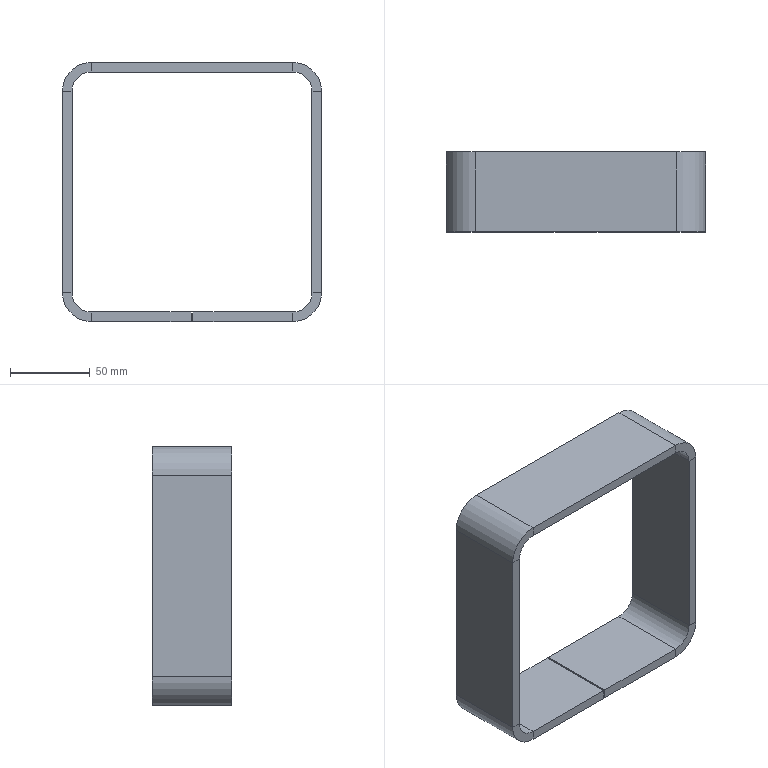Part | SolidWorks | features FlatPattern 1, SMBaseFlange 1, SheetMetal 1 | 1 solid | 38 faces | box 162 x 50 x 162 mm | volume 179174 mm3 | plane 30 | cylinder 8 | commonest cylinder face diameters 24 x4 36 x4
STEP:
#1=CARTESIAN_POINT('',(-63.,25.,-81.));
#2=VERTEX_POINT('',#1);
#3=CARTESIAN_POINT('',(-63.,25.,-75.));
#4=VERTEX_POINT('',#3);
#5=CARTESIAN_POINT('',(-63.,25.,-81.));
#6=DIRECTION('',(0.,0.,1.));
#7=VECTOR('',#6,1000.);
#8=LINE('',#5,#7);
#9=EDGE_CURVE('',#2,#4,#8,.T.);
#10=ORIENTED_EDGE('',*,*,#9,.F.);
#11=CARTESIAN_POINT('',(-81.,25.,-63.));
#12=VERTEX_POINT('',#11);
#13=CARTESIAN_POINT('',(-63.,25.,-63.));
#14=DIRECTION('',(0.,-1.,0.));
#15=DIRECTION('',(0.,0.,1.));
#16=AXIS2_PLACEMENT_3D('',#13,#14,#15);
#17=CIRCLE('',#16,18.);
#18=EDGE_CURVE('',#12,#2,#17,.T.);
#19=ORIENTED_EDGE('',*,*,#18,.F.);
#20=CARTESIAN_POINT('',(-75.,25.,-63.));
#21=VERTEX_POINT('',#20);
#22=CARTESIAN_POINT('',(-75.,25.,-63.));
#23=DIRECTION('',(-1.,0.,0.));
#24=VECTOR('',#23,1000.);
#25=LINE('',#22,#24);
#26=EDGE_CURVE('',#21,#12,#25,.T.);
#27=ORIENTED_EDGE('',*,*,#26,.F.);
#28=CARTESIAN_POINT('',(-63.,25.,-63.));
#29=DIRECTION('',(0.,-1.,0.));
#30=DIRECTION('',(1.,0.,0.));
#31=AXIS2_PLACEMENT_3D('',#28,#29,#30);
#32=CIRCLE('',#31,12.);
#33=EDGE_CURVE('',#21,#4,#32,.T.);
#34=ORIENTED_EDGE('',*,*,#33,.T.);
#35=EDGE_LOOP('',(#10,#19,#27,#34));
#36=FACE_OUTER_BOUND('',#35,.T.);
#37=CARTESIAN_POINT('',(-63.,25.,-81.));
#38=DIRECTION('',(0.,1.,0.));
#39=DIRECTION('',(0.,0.,1.));
#40=AXIS2_PLACEMENT_3D('',#37,#38,#39);
#41=PLANE('',#40);
#42=ADVANCED_FACE('',(#36),#41,.T.);
#43=CARTESIAN_POINT('',(-0.5,25.,-81.));
#44=VERTEX_POINT('',#43);
#45=CARTESIAN_POINT('',(-63.,25.,-81.));
#46=DIRECTION('',(1.,0.,0.));
#47=VECTOR('',#46,1000.);
#48=LINE('',#45,#47);
#49=EDGE_CURVE('',#2,#44,#48,.T.);
#50=ORIENTED_EDGE('',*,*,#49,.F.);
#51=ORIENTED_EDGE('',*,*,#9,.T.);
#52=CARTESIAN_POINT('',(-0.5,25.,-75.));
#53=VERTEX_POINT('',#52);
#54=CARTESIAN_POINT('',(-63.,25.,-75.));
#55=DIRECTION('',(1.,0.,0.));
#56=VECTOR('',#55,1000.);
#57=LINE('',#54,#56);
#58=EDGE_CURVE('',#4,#53,#57,.T.);
#59=ORIENTED_EDGE('',*,*,#58,.T.);
#60=CARTESIAN_POINT('',(-0.5,25.,-81.));
#61=DIRECTION('',(0.,0.,1.));
#62=VECTOR('',#61,1000.);
#63=LINE('',#60,#62);
#64=EDGE_CURVE('',#44,#53,#63,.T.);
#65=ORIENTED_EDGE('',*,*,#64,.F.);
#66=EDGE_LOOP('',(#50,#51,#59,#65));
#67=FACE_OUTER_BOUND('',#66,.T.);
#68=CARTESIAN_POINT('',(-75.,25.,-63.));
#69=DIRECTION('',(0.,1.,0.));
#70=DIRECTION('',(0.,0.,1.));
#71=AXIS2_PLACEMENT_3D('',#68,#69,#70);
#72=PLANE('',#71);
#73=ADVANCED_FACE('',(#67),#72,.T.);
#74=CARTESIAN_POINT('',(-81.,-25.,-63.));
#75=VERTEX_POINT('',#74);
#76=CARTESIAN_POINT('',(-75.,-25.,-63.));
#77=VERTEX_POINT('',#76);
#78=CARTESIAN_POINT('',(-81.,-25.,-63.));
#79=DIRECTION('',(1.,0.,0.));
#80=VECTOR('',#79,1000.);
#81=LINE('',#78,#80);
#82=EDGE_CURVE('',#75,#77,#81,.T.);
#83=ORIENTED_EDGE('',*,*,#82,.F.);
#84=CARTESIAN_POINT('',(-63.,-25.,-81.));
#85=VERTEX_POINT('',#84);
#86=CARTESIAN_POINT('',(-63.,-25.,-63.));
#87=DIRECTION('',(0.,-1.,0.));
#88=DIRECTION('',(0.,0.,1.));
#89=AXIS2_PLACEMENT_3D('',#86,#87,#88);
#90=CIRCLE('',#89,18.);
#91=EDGE_CURVE('',#75,#85,#90,.T.);
#92=ORIENTED_EDGE('',*,*,#91,.T.);
#93=CARTESIAN_POINT('',(-63.,-25.,-75.));
#94=VERTEX_POINT('',#93);
#95=CARTESIAN_POINT('',(-63.,-25.,-75.));
#96=DIRECTION('',(0.,0.,-1.));
#97=VECTOR('',#96,1000.);
#98=LINE('',#95,#97);
#99=EDGE_CURVE('',#94,#85,#98,.T.);
#100=ORIENTED_EDGE('',*,*,#99,.F.);
#101=CARTESIAN_POINT('',(-63.,-25.,-63.));
#102=DIRECTION('',(0.,-1.,0.));
#103=DIRECTION('',(1.,0.,0.));
#104=AXIS2_PLACEMENT_3D('',#101,#102,#103);
#105=CIRCLE('',#104,12.);
#106=EDGE_CURVE('',#77,#94,#105,.T.);
#107=ORIENTED_EDGE('',*,*,#106,.F.);
#108=EDGE_LOOP('',(#83,#92,#100,#107));
#109=FACE_OUTER_BOUND('',#108,.T.);
#110=CARTESIAN_POINT('',(-81.,-25.,-63.));
#111=DIRECTION('',(0.,-1.,0.));
#112=DIRECTION('',(0.,0.,-1.));
#113=AXIS2_PLACEMENT_3D('',#110,#111,#112);
#114=PLANE('',#113);
#115=ADVANCED_FACE('',(#109),#114,.T.);
#116=CARTESIAN_POINT('',(-81.,-25.,63.));
#117=VERTEX_POINT('',#116);
#118=CARTESIAN_POINT('',(-81.,-25.,-63.));
#119=DIRECTION('',(0.,0.,-1.));
#120=VECTOR('',#119,1000.);
#121=LINE('',#118,#120);
#122=EDGE_CURVE('',#117,#75,#121,.T.);
#123=ORIENTED_EDGE('',*,*,#122,.T.);
#124=ORIENTED_EDGE('',*,*,#82,.T.);
#125=CARTESIAN_POINT('',(-75.,-25.,63.));
#126=VERTEX_POINT('',#125);
#127=CARTESIAN_POINT('',(-75.,-25.,-63.));
#128=DIRECTION('',(0.,0.,-1.));
#129=VECTOR('',#128,1000.);
#130=LINE('',#127,#129);
#131=EDGE_CURVE('',#126,#77,#130,.T.);
#132=ORIENTED_EDGE('',*,*,#131,.F.);
#133=CARTESIAN_POINT('',(-75.,-25.,63.));
#134=DIRECTION('',(-1.,0.,0.));
#135=VECTOR('',#134,1000.);
#136=LINE('',#133,#135);
#137=EDGE_CURVE('',#126,#117,#136,.T.);
#138=ORIENTED_EDGE('',*,*,#137,.T.);
#139=EDGE_LOOP('',(#123,#124,#132,#138));
#140=FACE_OUTER_BOUND('',#139,.T.);
#141=CARTESIAN_POINT('',(-63.,-25.,-75.));
#142=DIRECTION('',(0.,-1.,0.));
#143=DIRECTION('',(0.,0.,-1.));
#144=AXIS2_PLACEMENT_3D('',#141,#142,#143);
#145=PLANE('',#144);
#146=ADVANCED_FACE('',(#140),#145,.T.);
#147=CARTESIAN_POINT('',(-81.,25.,63.));
#148=VERTEX_POINT('',#147);
#149=CARTESIAN_POINT('',(-75.,25.,63.));
#150=VERTEX_POINT('',#149);
#151=CARTESIAN_POINT('',(-81.,25.,63.));
#152=DIRECTION('',(1.,0.,0.));
#153=VECTOR('',#152,1000.);
#154=LINE('',#151,#153);
#155=EDGE_CURVE('',#148,#150,#154,.T.);
#156=ORIENTED_EDGE('',*,*,#155,.F.);
#157=CARTESIAN_POINT('',(-63.,25.,81.));
#158=VERTEX_POINT('',#157);
#159=CARTESIAN_POINT('',(-63.,25.,63.));
#160=DIRECTION('',(0.,-1.,0.));
#161=DIRECTION('',(0.,0.,1.));
#162=AXIS2_PLACEMENT_3D('',#159,#160,#161);
#163=CIRCLE('',#162,18.);
#164=EDGE_CURVE('',#158,#148,#163,.T.);
#165=ORIENTED_EDGE('',*,*,#164,.F.);
#166=CARTESIAN_POINT('',(-63.,25.,75.));
#167=VERTEX_POINT('',#166);
#168=CARTESIAN_POINT('',(-63.,25.,75.));
#169=DIRECTION('',(0.,0.,1.));
#170=VECTOR('',#169,1000.);
#171=LINE('',#168,#170);
#172=EDGE_CURVE('',#167,#158,#171,.T.);
#173=ORIENTED_EDGE('',*,*,#172,.F.);
#174=CARTESIAN_POINT('',(-63.,25.,63.));
#175=DIRECTION('',(0.,-1.,0.));
#176=DIRECTION('',(1.,0.,0.));
#177=AXIS2_PLACEMENT_3D('',#174,#175,#176);
#178=CIRCLE('',#177,12.);
#179=EDGE_CURVE('',#167,#150,#178,.T.);
#180=ORIENTED_EDGE('',*,*,#179,.T.);
#181=EDGE_LOOP('',(#156,#165,#173,#180));
#182=FACE_OUTER_BOUND('',#181,.T.);
#183=CARTESIAN_POINT('',(-81.,25.,63.));
#184=DIRECTION('',(0.,1.,0.));
#185=DIRECTION('',(0.,0.,1.));
#186=AXIS2_PLACEMENT_3D('',#183,#184,#185);
#187=PLANE('',#186);
#188=ADVANCED_FACE('',(#182),#187,.T.);
#189=CARTESIAN_POINT('',(-81.,25.,-63.));
#190=DIRECTION('',(0.,0.,-1.));
#191=VECTOR('',#190,1000.);
#192=LINE('',#189,#191);
#193=EDGE_CURVE('',#148,#12,#192,.T.);
#194=ORIENTED_EDGE('',*,*,#193,.F.);
#195=ORIENTED_EDGE('',*,*,#155,.T.);
#196=CARTESIAN_POINT('',(-75.,25.,-63.));
#197=DIRECTION('',(0.,0.,-1.));
#198=VECTOR('',#197,1000.);
#199=LINE('',#196,#198);
#200=EDGE_CURVE('',#150,#21,#199,.T.);
#201=ORIENTED_EDGE('',*,*,#200,.T.);
#202=ORIENTED_EDGE('',*,*,#26,.T.);
#203=EDGE_LOOP('',(#194,#195,#201,#202));
#204=FACE_OUTER_BOUND('',#203,.T.);
#205=CARTESIAN_POINT('',(-63.,25.,75.));
#206=DIRECTION('',(0.,1.,0.));
#207=DIRECTION('',(0.,0.,1.));
#208=AXIS2_PLACEMENT_3D('',#205,#206,#207);
#209=PLANE('',#208);
#210=ADVANCED_FACE('',(#204),#209,.T.);
#211=CARTESIAN_POINT('',(-63.,-25.,81.));
#212=VERTEX_POINT('',#211);
#213=CARTESIAN_POINT('',(-63.,-25.,75.));
#214=VERTEX_POINT('',#213);
#215=CARTESIAN_POINT('',(-63.,-25.,81.));
#216=DIRECTION('',(0.,0.,-1.));
#217=VECTOR('',#216,1000.);
#218=LINE('',#215,#217);
#219=EDGE_CURVE('',#212,#214,#218,.T.);
#220=ORIENTED_EDGE('',*,*,#219,.F.);
#221=CARTESIAN_POINT('',(-63.,-25.,63.));
#222=DIRECTION('',(0.,-1.,0.));
#223=DIRECTION('',(0.,0.,1.));
#224=AXIS2_PLACEMENT_3D('',#221,#222,#223);
#225=CIRCLE('',#224,18.);
#226=EDGE_CURVE('',#212,#117,#225,.T.);
#227=ORIENTED_EDGE('',*,*,#226,.T.);
#228=ORIENTED_EDGE('',*,*,#137,.F.);
#229=CARTESIAN_POINT('',(-63.,-25.,63.));
#230=DIRECTION('',(0.,-1.,0.));
#231=DIRECTION('',(1.,0.,0.));
#232=AXIS2_PLACEMENT_3D('',#229,#230,#231);
#233=CIRCLE('',#232,12.);
#234=EDGE_CURVE('',#214,#126,#233,.T.);
#235=ORIENTED_EDGE('',*,*,#234,.F.);
#236=EDGE_LOOP('',(#220,#227,#228,#235));
#237=FACE_OUTER_BOUND('',#236,.T.);
#238=CARTESIAN_POINT('',(-63.,-25.,81.));
#239=DIRECTION('',(0.,-1.,0.));
#240=DIRECTION('',(0.,0.,-1.));
#241=AXIS2_PLACEMENT_3D('',#238,#239,#240);
#242=PLANE('',#241);
#243=ADVANCED_FACE('',(#237),#242,.T.);
#244=CARTESIAN_POINT('',(63.,-25.,81.));
#245=VERTEX_POINT('',#244);
#246=CARTESIAN_POINT('',(-63.,-25.,81.));
#247=DIRECTION('',(-1.,0.,0.));
#248=VECTOR('',#247,1000.);
#249=LINE('',#246,#248);
#250=EDGE_CURVE('',#245,#212,#249,.T.);
#251=ORIENTED_EDGE('',*,*,#250,.T.);
#252=ORIENTED_EDGE('',*,*,#219,.T.);
#253=CARTESIAN_POINT('',(63.,-25.,75.));
#254=VERTEX_POINT('',#253);
#255=CARTESIAN_POINT('',(-63.,-25.,75.));
#256=DIRECTION('',(-1.,0.,0.));
#257=VECTOR('',#256,1000.);
#258=LINE('',#255,#257);
#259=EDGE_CURVE('',#254,#214,#258,.T.);
#260=ORIENTED_EDGE('',*,*,#259,.F.);
#261=CARTESIAN_POINT('',(63.,-25.,75.));
#262=DIRECTION('',(0.,0.,1.));
#263=VECTOR('',#262,1000.);
#264=LINE('',#261,#263);
#265=EDGE_CURVE('',#254,#245,#264,.T.);
#266=ORIENTED_EDGE('',*,*,#265,.T.);
#267=EDGE_LOOP('',(#251,#252,#260,#266));
#268=FACE_OUTER_BOUND('',#267,.T.);
#269=CARTESIAN_POINT('',(-75.,-25.,63.));
#270=DIRECTION('',(0.,-1.,0.));
#271=DIRECTION('',(0.,0.,-1.));
#272=AXIS2_PLACEMENT_3D('',#269,#270,#271);
#273=PLANE('',#272);
#274=ADVANCED_FACE('',(#268),#273,.T.);
#275=CARTESIAN_POINT('',(63.,25.,81.));
#276=VERTEX_POINT('',#275);
#277=CARTESIAN_POINT('',(63.,25.,75.));
#278=VERTEX_POINT('',#277);
#279=CARTESIAN_POINT('',(63.,25.,81.));
#280=DIRECTION('',(0.,0.,-1.));
#281=VECTOR('',#280,1000.);
#282=LINE('',#279,#281);
#283=EDGE_CURVE('',#276,#278,#282,.T.);
#284=ORIENTED_EDGE('',*,*,#283,.F.);
#285=CARTESIAN_POINT('',(81.,25.,63.));
#286=VERTEX_POINT('',#285);
#287=CARTESIAN_POINT('',(63.,25.,63.));
#288=DIRECTION('',(0.,-1.,0.));
#289=DIRECTION('',(0.,0.,1.));
#290=AXIS2_PLACEMENT_3D('',#287,#288,#289);
#291=CIRCLE('',#290,18.);
#292=EDGE_CURVE('',#286,#276,#291,.T.);
#293=ORIENTED_EDGE('',*,*,#292,.F.);
#294=CARTESIAN_POINT('',(75.,25.,63.));
#295=VERTEX_POINT('',#294);
#296=CARTESIAN_POINT('',(75.,25.,63.));
#297=DIRECTION('',(1.,0.,0.));
#298=VECTOR('',#297,1000.);
#299=LINE('',#296,#298);
#300=EDGE_CURVE('',#295,#286,#299,.T.);
#301=ORIENTED_EDGE('',*,*,#300,.F.);
#302=CARTESIAN_POINT('',(63.,25.,63.));
#303=DIRECTION('',(0.,-1.,0.));
#304=DIRECTION('',(1.,0.,0.));
#305=AXIS2_PLACEMENT_3D('',#302,#303,#304);
#306=CIRCLE('',#305,12.);
#307=EDGE_CURVE('',#295,#278,#306,.T.);
#308=ORIENTED_EDGE('',*,*,#307,.T.);
#309=EDGE_LOOP('',(#284,#293,#301,#308));
#310=FACE_OUTER_BOUND('',#309,.T.);
#311=CARTESIAN_POINT('',(63.,25.,81.));
#312=DIRECTION('',(0.,1.,0.));
#313=DIRECTION('',(0.,0.,1.));
#314=AXIS2_PLACEMENT_3D('',#311,#312,#313);
#315=PLANE('',#314);
#316=ADVANCED_FACE('',(#310),#315,.T.);
#317=CARTESIAN_POINT('',(-63.,25.,81.));
#318=DIRECTION('',(-1.,0.,0.));
#319=VECTOR('',#318,1000.);
#320=LINE('',#317,#319);
#321=EDGE_CURVE('',#276,#158,#320,.T.);
#322=ORIENTED_EDGE('',*,*,#321,.F.);
#323=ORIENTED_EDGE('',*,*,#283,.T.);
#324=CARTESIAN_POINT('',(-63.,25.,75.));
#325=DIRECTION('',(-1.,0.,0.));
#326=VECTOR('',#325,1000.);
#327=LINE('',#324,#326);
#328=EDGE_CURVE('',#278,#167,#327,.T.);
#329=ORIENTED_EDGE('',*,*,#328,.T.);
#330=ORIENTED_EDGE('',*,*,#172,.T.);
#331=EDGE_LOOP('',(#322,#323,#329,#330));
#332=FACE_OUTER_BOUND('',#331,.T.);
#333=CARTESIAN_POINT('',(75.,25.,63.));
#334=DIRECTION('',(0.,1.,0.));
#335=DIRECTION('',(0.,0.,1.));
#336=AXIS2_PLACEMENT_3D('',#333,#334,#335);
#337=PLANE('',#336);
#338=ADVANCED_FACE('',(#332),#337,.T.);
#339=CARTESIAN_POINT('',(81.,-25.,63.));
#340=VERTEX_POINT('',#339);
#341=CARTESIAN_POINT('',(75.,-25.,63.));
#342=VERTEX_POINT('',#341);
#343=CARTESIAN_POINT('',(81.,-25.,63.));
#344=DIRECTION('',(-1.,0.,0.));
#345=VECTOR('',#344,1000.);
#346=LINE('',#343,#345);
#347=EDGE_CURVE('',#340,#342,#346,.T.);
#348=ORIENTED_EDGE('',*,*,#347,.F.);
#349=CARTESIAN_POINT('',(63.,-25.,63.));
#350=DIRECTION('',(0.,-1.,0.));
#351=DIRECTION('',(0.,0.,1.));
#352=AXIS2_PLACEMENT_3D('',#349,#350,#351);
#353=CIRCLE('',#352,18.);
#354=EDGE_CURVE('',#340,#245,#353,.T.);
#355=ORIENTED_EDGE('',*,*,#354,.T.);
#356=ORIENTED_EDGE('',*,*,#265,.F.);
#357=CARTESIAN_POINT('',(63.,-25.,63.));
#358=DIRECTION('',(0.,-1.,0.));
#359=DIRECTION('',(1.,0.,0.));
#360=AXIS2_PLACEMENT_3D('',#357,#358,#359);
#361=CIRCLE('',#360,12.);
#362=EDGE_CURVE('',#342,#254,#361,.T.);
#363=ORIENTED_EDGE('',*,*,#362,.F.);
#364=EDGE_LOOP('',(#348,#355,#356,#363));
#365=FACE_OUTER_BOUND('',#364,.T.);
#366=CARTESIAN_POINT('',(81.,-25.,63.));
#367=DIRECTION('',(0.,-1.,0.));
#368=DIRECTION('',(0.,0.,-1.));
#369=AXIS2_PLACEMENT_3D('',#366,#367,#368);
#370=PLANE('',#369);
#371=ADVANCED_FACE('',(#365),#370,.T.);
#372=CARTESIAN_POINT('',(81.,-25.,-63.));
#373=VERTEX_POINT('',#372);
#374=CARTESIAN_POINT('',(81.,-25.,-63.));
#375=DIRECTION('',(0.,0.,1.));
#376=VECTOR('',#375,1000.);
#377=LINE('',#374,#376);
#378=EDGE_CURVE('',#373,#340,#377,.T.);
#379=ORIENTED_EDGE('',*,*,#378,.T.);
#380=ORIENTED_EDGE('',*,*,#347,.T.);
#381=CARTESIAN_POINT('',(75.,-25.,-63.));
#382=VERTEX_POINT('',#381);
#383=CARTESIAN_POINT('',(75.,-25.,-63.));
#384=DIRECTION('',(0.,0.,1.));
#385=VECTOR('',#384,1000.);
#386=LINE('',#383,#385);
#387=EDGE_CURVE('',#382,#342,#386,.T.);
#388=ORIENTED_EDGE('',*,*,#387,.F.);
#389=CARTESIAN_POINT('',(75.,-25.,-63.));
#390=DIRECTION('',(1.,0.,0.));
#391=VECTOR('',#390,1000.);
#392=LINE('',#389,#391);
#393=EDGE_CURVE('',#382,#373,#392,.T.);
#394=ORIENTED_EDGE('',*,*,#393,.T.);
#395=EDGE_LOOP('',(#379,#380,#388,#394));
#396=FACE_OUTER_BOUND('',#395,.T.);
#397=CARTESIAN_POINT('',(63.,-25.,75.));
#398=DIRECTION('',(0.,-1.,0.));
#399=DIRECTION('',(0.,0.,-1.));
#400=AXIS2_PLACEMENT_3D('',#397,#398,#399);
#401=PLANE('',#400);
#402=ADVANCED_FACE('',(#396),#401,.T.);
#403=CARTESIAN_POINT('',(81.,25.,-63.));
#404=VERTEX_POINT('',#403);
#405=CARTESIAN_POINT('',(75.,25.,-63.));
#406=VERTEX_POINT('',#405);
#407=CARTESIAN_POINT('',(81.,25.,-63.));
#408=DIRECTION('',(-1.,0.,0.));
#409=VECTOR('',#408,1000.);
#410=LINE('',#407,#409);
#411=EDGE_CURVE('',#404,#406,#410,.T.);
#412=ORIENTED_EDGE('',*,*,#411,.F.);
#413=CARTESIAN_POINT('',(63.,25.,-81.));
#414=VERTEX_POINT('',#413);
#415=CARTESIAN_POINT('',(63.,25.,-63.));
#416=DIRECTION('',(0.,-1.,0.));
#417=DIRECTION('',(0.,0.,-1.));
#418=AXIS2_PLACEMENT_3D('',#415,#416,#417);
#419=CIRCLE('',#418,18.);
#420=EDGE_CURVE('',#414,#404,#419,.T.);
#421=ORIENTED_EDGE('',*,*,#420,.F.);
#422=CARTESIAN_POINT('',(63.,25.,-75.));
#423=VERTEX_POINT('',#422);
#424=CARTESIAN_POINT('',(63.,25.,-75.));
#425=DIRECTION('',(0.,0.,-1.));
#426=VECTOR('',#425,1000.);
#427=LINE('',#424,#426);
#428=EDGE_CURVE('',#423,#414,#427,.T.);
#429=ORIENTED_EDGE('',*,*,#428,.F.);
#430=CARTESIAN_POINT('',(63.,25.,-63.));
#431=DIRECTION('',(0.,-1.,0.));
#432=DIRECTION('',(1.,0.,0.));
#433=AXIS2_PLACEMENT_3D('',#430,#431,#432);
#434=CIRCLE('',#433,12.);
#435=EDGE_CURVE('',#423,#406,#434,.T.);
#436=ORIENTED_EDGE('',*,*,#435,.T.);
#437=EDGE_LOOP('',(#412,#421,#429,#436));
#438=FACE_OUTER_BOUND('',#437,.T.);
#439=CARTESIAN_POINT('',(81.,25.,-63.));
#440=DIRECTION('',(0.,1.,0.));
#441=DIRECTION('',(0.,0.,1.));
#442=AXIS2_PLACEMENT_3D('',#439,#440,#441);
#443=PLANE('',#442);
#444=ADVANCED_FACE('',(#438),#443,.T.);
#445=CARTESIAN_POINT('',(81.,25.,-63.));
#446=DIRECTION('',(0.,0.,1.));
#447=VECTOR('',#446,1000.);
#448=LINE('',#445,#447);
#449=EDGE_CURVE('',#404,#286,#448,.T.);
#450=ORIENTED_EDGE('',*,*,#449,.F.);
#451=ORIENTED_EDGE('',*,*,#411,.T.);
#452=CARTESIAN_POINT('',(75.,25.,-63.));
#453=DIRECTION('',(0.,0.,1.));
#454=VECTOR('',#453,1000.);
#455=LINE('',#452,#454);
#456=EDGE_CURVE('',#406,#295,#455,.T.);
#457=ORIENTED_EDGE('',*,*,#456,.T.);
#458=ORIENTED_EDGE('',*,*,#300,.T.);
#459=EDGE_LOOP('',(#450,#451,#457,#458));
#460=FACE_OUTER_BOUND('',#459,.T.);
#461=CARTESIAN_POINT('',(63.,25.,-75.));
#462=DIRECTION('',(0.,1.,0.));
#463=DIRECTION('',(0.,0.,1.));
#464=AXIS2_PLACEMENT_3D('',#461,#462,#463);
#465=PLANE('',#464);
#466=ADVANCED_FACE('',(#460),#465,.T.);
#467=CARTESIAN_POINT('',(63.,-25.,-81.));
#468=VERTEX_POINT('',#467);
#469=CARTESIAN_POINT('',(63.,-25.,-75.));
#470=VERTEX_POINT('',#469);
#471=CARTESIAN_POINT('',(63.,-25.,-81.));
#472=DIRECTION('',(0.,0.,1.));
#473=VECTOR('',#472,1000.);
#474=LINE('',#471,#473);
#475=EDGE_CURVE('',#468,#470,#474,.T.);
#476=ORIENTED_EDGE('',*,*,#475,.F.);
#477=CARTESIAN_POINT('',(63.,-25.,-63.));
#478=DIRECTION('',(0.,-1.,0.));
#479=DIRECTION('',(0.,0.,-1.));
#480=AXIS2_PLACEMENT_3D('',#477,#478,#479);
#481=CIRCLE('',#480,18.);
#482=EDGE_CURVE('',#468,#373,#481,.T.);
#483=ORIENTED_EDGE('',*,*,#482,.T.);
#484=ORIENTED_EDGE('',*,*,#393,.F.);
#485=CARTESIAN_POINT('',(63.,-25.,-63.));
#486=DIRECTION('',(0.,-1.,0.));
#487=DIRECTION('',(1.,0.,0.));
#488=AXIS2_PLACEMENT_3D('',#485,#486,#487);
#489=CIRCLE('',#488,12.);
#490=EDGE_CURVE('',#470,#382,#489,.T.);
#491=ORIENTED_EDGE('',*,*,#490,.F.);
#492=EDGE_LOOP('',(#476,#483,#484,#491));
#493=FACE_OUTER_BOUND('',#492,.T.);
#494=CARTESIAN_POINT('',(63.,-25.,-81.));
#495=DIRECTION('',(0.,-1.,0.));
#496=DIRECTION('',(0.,0.,-1.));
#497=AXIS2_PLACEMENT_3D('',#494,#495,#496);
#498=PLANE('',#497);
#499=ADVANCED_FACE('',(#493),#498,.T.);
#500=CARTESIAN_POINT('',(0.5,-25.,-81.));
#501=VERTEX_POINT('',#500);
#502=CARTESIAN_POINT('',(0.5,-25.,-81.));
#503=DIRECTION('',(1.,0.,0.));
#504=VECTOR('',#503,1000.);
#505=LINE('',#502,#504);
#506=EDGE_CURVE('',#501,#468,#505,.T.);
#507=ORIENTED_EDGE('',*,*,#506,.T.);
#508=ORIENTED_EDGE('',*,*,#475,.T.);
#509=CARTESIAN_POINT('',(0.5,-25.,-75.));
#510=VERTEX_POINT('',#509);
#511=CARTESIAN_POINT('',(0.5,-25.,-75.));
#512=DIRECTION('',(1.,0.,0.));
#513=VECTOR('',#512,1000.);
#514=LINE('',#511,#513);
#515=EDGE_CURVE('',#510,#470,#514,.T.);
#516=ORIENTED_EDGE('',*,*,#515,.F.);
#517=CARTESIAN_POINT('',(0.5,-25.,-75.));
#518=DIRECTION('',(0.,0.,-1.));
#519=VECTOR('',#518,1000.);
#520=LINE('',#517,#519);
#521=EDGE_CURVE('',#510,#501,#520,.T.);
#522=ORIENTED_EDGE('',*,*,#521,.T.);
#523=EDGE_LOOP('',(#507,#508,#516,#522));
#524=FACE_OUTER_BOUND('',#523,.T.);
#525=CARTESIAN_POINT('',(75.,-25.,-63.));
#526=DIRECTION('',(0.,-1.,0.));
#527=DIRECTION('',(0.,0.,-1.));
#528=AXIS2_PLACEMENT_3D('',#525,#526,#527);
#529=PLANE('',#528);
#530=ADVANCED_FACE('',(#524),#529,.T.);
#531=CARTESIAN_POINT('',(-0.5,-25.,-75.));
#532=VERTEX_POINT('',#531);
#533=CARTESIAN_POINT('',(-63.,-25.,-75.));
#534=DIRECTION('',(1.,0.,0.));
#535=VECTOR('',#534,1000.);
#536=LINE('',#533,#535);
#537=EDGE_CURVE('',#94,#532,#536,.T.);
#538=ORIENTED_EDGE('',*,*,#537,.T.);
#539=CARTESIAN_POINT('',(-0.5,25.,-75.));
#540=DIRECTION('',(0.,-1.,0.));
#541=VECTOR('',#540,1000.);
#542=LINE('',#539,#541);
#543=EDGE_CURVE('',#53,#532,#542,.T.);
#544=ORIENTED_EDGE('',*,*,#543,.F.);
#545=ORIENTED_EDGE('',*,*,#58,.F.);
#546=CARTESIAN_POINT('',(-63.,25.,-75.));
#547=DIRECTION('',(0.,-1.,0.));
#548=VECTOR('',#547,1000.);
#549=LINE('',#546,#548);
#550=EDGE_CURVE('',#4,#94,#549,.T.);
#551=ORIENTED_EDGE('',*,*,#550,.T.);
#552=EDGE_LOOP('',(#538,#544,#545,#551));
#553=FACE_OUTER_BOUND('',#552,.T.);
#554=CARTESIAN_POINT('',(-63.,25.,-75.));
#555=DIRECTION('',(0.,0.,-1.));
#556=DIRECTION('',(-1.,0.,0.));
#557=AXIS2_PLACEMENT_3D('',#554,#555,#556);
#558=PLANE('',#557);
#559=ADVANCED_FACE('',(#553),#558,.F.);
#560=CARTESIAN_POINT('',(-0.5,-25.,-81.));
#561=VERTEX_POINT('',#560);
#562=CARTESIAN_POINT('',(-0.5,-25.,-81.));
#563=DIRECTION('',(0.,0.,1.));
#564=VECTOR('',#563,1000.);
#565=LINE('',#562,#564);
#566=EDGE_CURVE('',#561,#532,#565,.T.);
#567=ORIENTED_EDGE('',*,*,#566,.F.);
#568=CARTESIAN_POINT('',(-0.5,25.,-81.));
#569=DIRECTION('',(0.,-1.,0.));
#570=VECTOR('',#569,1000.);
#571=LINE('',#568,#570);
#572=EDGE_CURVE('',#44,#561,#571,.T.);
#573=ORIENTED_EDGE('',*,*,#572,.F.);
#574=ORIENTED_EDGE('',*,*,#64,.T.);
#575=ORIENTED_EDGE('',*,*,#543,.T.);
#576=EDGE_LOOP('',(#567,#573,#574,#575));
#577=FACE_OUTER_BOUND('',#576,.T.);
#578=CARTESIAN_POINT('',(-0.5,25.,-81.));
#579=DIRECTION('',(1.,0.,0.));
#580=DIRECTION('',(0.,0.,-1.));
#581=AXIS2_PLACEMENT_3D('',#578,#579,#580);
#582=PLANE('',#581);
#583=ADVANCED_FACE('',(#577),#582,.T.);
#584=CARTESIAN_POINT('',(-63.,-25.,-81.));
#585=DIRECTION('',(1.,0.,0.));
#586=VECTOR('',#585,1000.);
#587=LINE('',#584,#586);
#588=EDGE_CURVE('',#85,#561,#587,.T.);
#589=ORIENTED_EDGE('',*,*,#588,.F.);
#590=CARTESIAN_POINT('',(-63.,25.,-81.));
#591=DIRECTION('',(0.,-1.,0.));
#592=VECTOR('',#591,1000.);
#593=LINE('',#590,#592);
#594=EDGE_CURVE('',#2,#85,#593,.T.);
#595=ORIENTED_EDGE('',*,*,#594,.F.);
#596=ORIENTED_EDGE('',*,*,#49,.T.);
#597=ORIENTED_EDGE('',*,*,#572,.T.);
#598=EDGE_LOOP('',(#589,#595,#596,#597));
#599=FACE_OUTER_BOUND('',#598,.T.);
#600=CARTESIAN_POINT('',(-63.,25.,-81.));
#601=DIRECTION('',(0.,0.,-1.));
#602=DIRECTION('',(-1.,0.,0.));
#603=AXIS2_PLACEMENT_3D('',#600,#601,#602);
#604=PLANE('',#603);
#605=ADVANCED_FACE('',(#599),#604,.T.);
#606=ORIENTED_EDGE('',*,*,#91,.F.);
#607=CARTESIAN_POINT('',(-81.,25.,-63.));
#608=DIRECTION('',(0.,-1.,0.));
#609=VECTOR('',#608,1000.);
#610=LINE('',#607,#609);
#611=EDGE_CURVE('',#12,#75,#610,.T.);
#612=ORIENTED_EDGE('',*,*,#611,.F.);
#613=ORIENTED_EDGE('',*,*,#18,.T.);
#614=ORIENTED_EDGE('',*,*,#594,.T.);
#615=EDGE_LOOP('',(#606,#612,#613,#614));
#616=FACE_OUTER_BOUND('',#615,.T.);
#617=CARTESIAN_POINT('',(-63.,25.,-63.));
#618=DIRECTION('',(0.,-1.,0.));
#619=DIRECTION('',(0.,0.,-1.));
#620=AXIS2_PLACEMENT_3D('',#617,#618,#619);
#621=CYLINDRICAL_SURFACE('',#620,18.);
#622=ADVANCED_FACE('',(#616),#621,.T.);
#623=ORIENTED_EDGE('',*,*,#122,.F.);
#624=CARTESIAN_POINT('',(-81.,25.,63.));
#625=DIRECTION('',(0.,-1.,0.));
#626=VECTOR('',#625,1000.);
#627=LINE('',#624,#626);
#628=EDGE_CURVE('',#148,#117,#627,.T.);
#629=ORIENTED_EDGE('',*,*,#628,.F.);
#630=ORIENTED_EDGE('',*,*,#193,.T.);
#631=ORIENTED_EDGE('',*,*,#611,.T.);
#632=EDGE_LOOP('',(#623,#629,#630,#631));
#633=FACE_OUTER_BOUND('',#632,.T.);
#634=CARTESIAN_POINT('',(-81.,25.,-63.));
#635=DIRECTION('',(-1.,0.,0.));
#636=DIRECTION('',(0.,0.,1.));
#637=AXIS2_PLACEMENT_3D('',#634,#635,#636);
#638=PLANE('',#637);
#639=ADVANCED_FACE('',(#633),#638,.T.);
#640=ORIENTED_EDGE('',*,*,#226,.F.);
#641=CARTESIAN_POINT('',(-63.,25.,81.));
#642=DIRECTION('',(0.,-1.,0.));
#643=VECTOR('',#642,1000.);
#644=LINE('',#641,#643);
#645=EDGE_CURVE('',#158,#212,#644,.T.);
#646=ORIENTED_EDGE('',*,*,#645,.F.);
#647=ORIENTED_EDGE('',*,*,#164,.T.);
#648=ORIENTED_EDGE('',*,*,#628,.T.);
#649=EDGE_LOOP('',(#640,#646,#647,#648));
#650=FACE_OUTER_BOUND('',#649,.T.);
#651=CARTESIAN_POINT('',(-63.,25.,63.));
#652=DIRECTION('',(0.,-1.,0.));
#653=DIRECTION('',(0.,0.,-1.));
#654=AXIS2_PLACEMENT_3D('',#651,#652,#653);
#655=CYLINDRICAL_SURFACE('',#654,18.);
#656=ADVANCED_FACE('',(#650),#655,.T.);
#657=ORIENTED_EDGE('',*,*,#250,.F.);
#658=CARTESIAN_POINT('',(63.,25.,81.));
#659=DIRECTION('',(0.,-1.,0.));
#660=VECTOR('',#659,1000.);
#661=LINE('',#658,#660);
#662=EDGE_CURVE('',#276,#245,#661,.T.);
#663=ORIENTED_EDGE('',*,*,#662,.F.);
#664=ORIENTED_EDGE('',*,*,#321,.T.);
#665=ORIENTED_EDGE('',*,*,#645,.T.);
#666=EDGE_LOOP('',(#657,#663,#664,#665));
#667=FACE_OUTER_BOUND('',#666,.T.);
#668=CARTESIAN_POINT('',(-63.,25.,81.));
#669=DIRECTION('',(0.,0.,1.));
#670=DIRECTION('',(1.,0.,0.));
#671=AXIS2_PLACEMENT_3D('',#668,#669,#670);
#672=PLANE('',#671);
#673=ADVANCED_FACE('',(#667),#672,.T.);
#674=ORIENTED_EDGE('',*,*,#354,.F.);
#675=CARTESIAN_POINT('',(81.,25.,63.));
#676=DIRECTION('',(0.,-1.,0.));
#677=VECTOR('',#676,1000.);
#678=LINE('',#675,#677);
#679=EDGE_CURVE('',#286,#340,#678,.T.);
#680=ORIENTED_EDGE('',*,*,#679,.F.);
#681=ORIENTED_EDGE('',*,*,#292,.T.);
#682=ORIENTED_EDGE('',*,*,#662,.T.);
#683=EDGE_LOOP('',(#674,#680,#681,#682));
#684=FACE_OUTER_BOUND('',#683,.T.);
#685=CARTESIAN_POINT('',(63.,25.,63.));
#686=DIRECTION('',(0.,-1.,0.));
#687=DIRECTION('',(0.,0.,-1.));
#688=AXIS2_PLACEMENT_3D('',#685,#686,#687);
#689=CYLINDRICAL_SURFACE('',#688,18.);
#690=ADVANCED_FACE('',(#684),#689,.T.);
#691=ORIENTED_EDGE('',*,*,#378,.F.);
#692=CARTESIAN_POINT('',(81.,25.,-63.));
#693=DIRECTION('',(0.,-1.,0.));
#694=VECTOR('',#693,1000.);
#695=LINE('',#692,#694);
#696=EDGE_CURVE('',#404,#373,#695,.T.);
#697=ORIENTED_EDGE('',*,*,#696,.F.);
#698=ORIENTED_EDGE('',*,*,#449,.T.);
#699=ORIENTED_EDGE('',*,*,#679,.T.);
#700=EDGE_LOOP('',(#691,#697,#698,#699));
#701=FACE_OUTER_BOUND('',#700,.T.);
#702=CARTESIAN_POINT('',(81.,25.,-63.));
#703=DIRECTION('',(1.,0.,0.));
#704=DIRECTION('',(0.,0.,-1.));
#705=AXIS2_PLACEMENT_3D('',#702,#703,#704);
#706=PLANE('',#705);
#707=ADVANCED_FACE('',(#701),#706,.T.);
#708=ORIENTED_EDGE('',*,*,#482,.F.);
#709=CARTESIAN_POINT('',(63.,25.,-81.));
#710=DIRECTION('',(0.,-1.,0.));
#711=VECTOR('',#710,1000.);
#712=LINE('',#709,#711);
#713=EDGE_CURVE('',#414,#468,#712,.T.);
#714=ORIENTED_EDGE('',*,*,#713,.F.);
#715=ORIENTED_EDGE('',*,*,#420,.T.);
#716=ORIENTED_EDGE('',*,*,#696,.T.);
#717=EDGE_LOOP('',(#708,#714,#715,#716));
#718=FACE_OUTER_BOUND('',#717,.T.);
#719=CARTESIAN_POINT('',(63.,25.,-63.));
#720=DIRECTION('',(0.,-1.,0.));
#721=DIRECTION('',(0.,0.,-1.));
#722=AXIS2_PLACEMENT_3D('',#719,#720,#721);
#723=CYLINDRICAL_SURFACE('',#722,18.);
#724=ADVANCED_FACE('',(#718),#723,.T.);
#725=ORIENTED_EDGE('',*,*,#506,.F.);
#726=CARTESIAN_POINT('',(0.5,25.,-81.));
#727=VERTEX_POINT('',#726);
#728=CARTESIAN_POINT('',(0.5,25.,-81.));
#729=DIRECTION('',(0.,-1.,0.));
#730=VECTOR('',#729,1000.);
#731=LINE('',#728,#730);
#732=EDGE_CURVE('',#727,#501,#731,.T.);
#733=ORIENTED_EDGE('',*,*,#732,.F.);
#734=CARTESIAN_POINT('',(0.5,25.,-81.));
#735=DIRECTION('',(1.,0.,0.));
#736=VECTOR('',#735,1000.);
#737=LINE('',#734,#736);
#738=EDGE_CURVE('',#727,#414,#737,.T.);
#739=ORIENTED_EDGE('',*,*,#738,.T.);
#740=ORIENTED_EDGE('',*,*,#713,.T.);
#741=EDGE_LOOP('',(#725,#733,#739,#740));
#742=FACE_OUTER_BOUND('',#741,.T.);
#743=CARTESIAN_POINT('',(0.5,25.,-81.));
#744=DIRECTION('',(0.,0.,-1.));
#745=DIRECTION('',(-1.,0.,0.));
#746=AXIS2_PLACEMENT_3D('',#743,#744,#745);
#747=PLANE('',#746);
#748=ADVANCED_FACE('',(#742),#747,.T.);
#749=ORIENTED_EDGE('',*,*,#521,.F.);
#750=CARTESIAN_POINT('',(0.5,25.,-75.));
#751=VERTEX_POINT('',#750);
#752=CARTESIAN_POINT('',(0.5,25.,-75.));
#753=DIRECTION('',(0.,-1.,0.));
#754=VECTOR('',#753,1000.);
#755=LINE('',#752,#754);
#756=EDGE_CURVE('',#751,#510,#755,.T.);
#757=ORIENTED_EDGE('',*,*,#756,.F.);
#758=CARTESIAN_POINT('',(0.5,25.,-75.));
#759=DIRECTION('',(0.,0.,-1.));
#760=VECTOR('',#759,1000.);
#761=LINE('',#758,#760);
#762=EDGE_CURVE('',#751,#727,#761,.T.);
#763=ORIENTED_EDGE('',*,*,#762,.T.);
#764=ORIENTED_EDGE('',*,*,#732,.T.);
#765=EDGE_LOOP('',(#749,#757,#763,#764));
#766=FACE_OUTER_BOUND('',#765,.T.);
#767=CARTESIAN_POINT('',(0.5,25.,-75.));
#768=DIRECTION('',(-1.,0.,0.));
#769=DIRECTION('',(0.,0.,1.));
#770=AXIS2_PLACEMENT_3D('',#767,#768,#769);
#771=PLANE('',#770);
#772=ADVANCED_FACE('',(#766),#771,.T.);
#773=ORIENTED_EDGE('',*,*,#515,.T.);
#774=CARTESIAN_POINT('',(63.,25.,-75.));
#775=DIRECTION('',(0.,-1.,0.));
#776=VECTOR('',#775,1000.);
#777=LINE('',#774,#776);
#778=EDGE_CURVE('',#423,#470,#777,.T.);
#779=ORIENTED_EDGE('',*,*,#778,.F.);
#780=CARTESIAN_POINT('',(0.5,25.,-75.));
#781=DIRECTION('',(1.,0.,0.));
#782=VECTOR('',#781,1000.);
#783=LINE('',#780,#782);
#784=EDGE_CURVE('',#751,#423,#783,.T.);
#785=ORIENTED_EDGE('',*,*,#784,.F.);
#786=ORIENTED_EDGE('',*,*,#756,.T.);
#787=EDGE_LOOP('',(#773,#779,#785,#786));
#788=FACE_OUTER_BOUND('',#787,.T.);
#789=CARTESIAN_POINT('',(0.5,25.,-75.));
#790=DIRECTION('',(0.,0.,-1.));
#791=DIRECTION('',(-1.,0.,0.));
#792=AXIS2_PLACEMENT_3D('',#789,#790,#791);
#793=PLANE('',#792);
#794=ADVANCED_FACE('',(#788),#793,.F.);
#795=ORIENTED_EDGE('',*,*,#490,.T.);
#796=CARTESIAN_POINT('',(75.,25.,-63.));
#797=DIRECTION('',(0.,-1.,0.));
#798=VECTOR('',#797,1000.);
#799=LINE('',#796,#798);
#800=EDGE_CURVE('',#406,#382,#799,.T.);
#801=ORIENTED_EDGE('',*,*,#800,.F.);
#802=ORIENTED_EDGE('',*,*,#435,.F.);
#803=ORIENTED_EDGE('',*,*,#778,.T.);
#804=EDGE_LOOP('',(#795,#801,#802,#803));
#805=FACE_OUTER_BOUND('',#804,.T.);
#806=CARTESIAN_POINT('',(63.,25.,-63.));
#807=DIRECTION('',(0.,-1.,0.));
#808=DIRECTION('',(0.,0.,-1.));
#809=AXIS2_PLACEMENT_3D('',#806,#807,#808);
#810=CYLINDRICAL_SURFACE('',#809,12.);
#811=ADVANCED_FACE('',(#805),#810,.F.);
#812=ORIENTED_EDGE('',*,*,#387,.T.);
#813=CARTESIAN_POINT('',(75.,25.,63.));
#814=DIRECTION('',(0.,-1.,0.));
#815=VECTOR('',#814,1000.);
#816=LINE('',#813,#815);
#817=EDGE_CURVE('',#295,#342,#816,.T.);
#818=ORIENTED_EDGE('',*,*,#817,.F.);
#819=ORIENTED_EDGE('',*,*,#456,.F.);
#820=ORIENTED_EDGE('',*,*,#800,.T.);
#821=EDGE_LOOP('',(#812,#818,#819,#820));
#822=FACE_OUTER_BOUND('',#821,.T.);
#823=CARTESIAN_POINT('',(75.,25.,-63.));
#824=DIRECTION('',(1.,0.,0.));
#825=DIRECTION('',(0.,0.,-1.));
#826=AXIS2_PLACEMENT_3D('',#823,#824,#825);
#827=PLANE('',#826);
#828=ADVANCED_FACE('',(#822),#827,.F.);
#829=ORIENTED_EDGE('',*,*,#362,.T.);
#830=CARTESIAN_POINT('',(63.,25.,75.));
#831=DIRECTION('',(0.,-1.,0.));
#832=VECTOR('',#831,1000.);
#833=LINE('',#830,#832);
#834=EDGE_CURVE('',#278,#254,#833,.T.);
#835=ORIENTED_EDGE('',*,*,#834,.F.);
#836=ORIENTED_EDGE('',*,*,#307,.F.);
#837=ORIENTED_EDGE('',*,*,#817,.T.);
#838=EDGE_LOOP('',(#829,#835,#836,#837));
#839=FACE_OUTER_BOUND('',#838,.T.);
#840=CARTESIAN_POINT('',(63.,25.,63.));
#841=DIRECTION('',(0.,-1.,0.));
#842=DIRECTION('',(0.,0.,-1.));
#843=AXIS2_PLACEMENT_3D('',#840,#841,#842);
#844=CYLINDRICAL_SURFACE('',#843,12.);
#845=ADVANCED_FACE('',(#839),#844,.F.);
#846=ORIENTED_EDGE('',*,*,#259,.T.);
#847=CARTESIAN_POINT('',(-63.,25.,75.));
#848=DIRECTION('',(0.,-1.,0.));
#849=VECTOR('',#848,1000.);
#850=LINE('',#847,#849);
#851=EDGE_CURVE('',#167,#214,#850,.T.);
#852=ORIENTED_EDGE('',*,*,#851,.F.);
#853=ORIENTED_EDGE('',*,*,#328,.F.);
#854=ORIENTED_EDGE('',*,*,#834,.T.);
#855=EDGE_LOOP('',(#846,#852,#853,#854));
#856=FACE_OUTER_BOUND('',#855,.T.);
#857=CARTESIAN_POINT('',(-63.,25.,75.));
#858=DIRECTION('',(0.,0.,1.));
#859=DIRECTION('',(1.,0.,0.));
#860=AXIS2_PLACEMENT_3D('',#857,#858,#859);
#861=PLANE('',#860);
#862=ADVANCED_FACE('',(#856),#861,.F.);
#863=ORIENTED_EDGE('',*,*,#234,.T.);
#864=CARTESIAN_POINT('',(-75.,25.,63.));
#865=DIRECTION('',(0.,-1.,0.));
#866=VECTOR('',#865,1000.);
#867=LINE('',#864,#866);
#868=EDGE_CURVE('',#150,#126,#867,.T.);
#869=ORIENTED_EDGE('',*,*,#868,.F.);
#870=ORIENTED_EDGE('',*,*,#179,.F.);
#871=ORIENTED_EDGE('',*,*,#851,.T.);
#872=EDGE_LOOP('',(#863,#869,#870,#871));
#873=FACE_OUTER_BOUND('',#872,.T.);
#874=CARTESIAN_POINT('',(-63.,25.,63.));
#875=DIRECTION('',(0.,-1.,0.));
#876=DIRECTION('',(0.,0.,-1.));
#877=AXIS2_PLACEMENT_3D('',#874,#875,#876);
#878=CYLINDRICAL_SURFACE('',#877,12.);
#879=ADVANCED_FACE('',(#873),#878,.F.);
#880=ORIENTED_EDGE('',*,*,#131,.T.);
#881=CARTESIAN_POINT('',(-75.,25.,-63.));
#882=DIRECTION('',(0.,-1.,0.));
#883=VECTOR('',#882,1000.);
#884=LINE('',#881,#883);
#885=EDGE_CURVE('',#21,#77,#884,.T.);
#886=ORIENTED_EDGE('',*,*,#885,.F.);
#887=ORIENTED_EDGE('',*,*,#200,.F.);
#888=ORIENTED_EDGE('',*,*,#868,.T.);
#889=EDGE_LOOP('',(#880,#886,#887,#888));
#890=FACE_OUTER_BOUND('',#889,.T.);
#891=CARTESIAN_POINT('',(-75.,25.,-63.));
#892=DIRECTION('',(-1.,0.,0.));
#893=DIRECTION('',(0.,0.,1.));
#894=AXIS2_PLACEMENT_3D('',#891,#892,#893);
#895=PLANE('',#894);
#896=ADVANCED_FACE('',(#890),#895,.F.);
#897=ORIENTED_EDGE('',*,*,#106,.T.);
#898=ORIENTED_EDGE('',*,*,#550,.F.);
#899=ORIENTED_EDGE('',*,*,#33,.F.);
#900=ORIENTED_EDGE('',*,*,#885,.T.);
#901=EDGE_LOOP('',(#897,#898,#899,#900));
#902=FACE_OUTER_BOUND('',#901,.T.);
#903=CARTESIAN_POINT('',(-63.,25.,-63.));
#904=DIRECTION('',(0.,-1.,0.));
#905=DIRECTION('',(0.,0.,-1.));
#906=AXIS2_PLACEMENT_3D('',#903,#904,#905);
#907=CYLINDRICAL_SURFACE('',#906,12.);
#908=ADVANCED_FACE('',(#902),#907,.F.);
#909=ORIENTED_EDGE('',*,*,#784,.T.);
#910=ORIENTED_EDGE('',*,*,#428,.T.);
#911=ORIENTED_EDGE('',*,*,#738,.F.);
#912=ORIENTED_EDGE('',*,*,#762,.F.);
#913=EDGE_LOOP('',(#909,#910,#911,#912));
#914=FACE_OUTER_BOUND('',#913,.T.);
#915=CARTESIAN_POINT('',(-63.,25.,-63.));
#916=DIRECTION('',(0.,-1.,0.));
#917=DIRECTION('',(-1.,0.,0.));
#918=AXIS2_PLACEMENT_3D('',#915,#916,#917);
#919=PLANE('',#918);
#920=ADVANCED_FACE('',(#914),#919,.F.);
#921=ORIENTED_EDGE('',*,*,#537,.F.);
#922=ORIENTED_EDGE('',*,*,#99,.T.);
#923=ORIENTED_EDGE('',*,*,#588,.T.);
#924=ORIENTED_EDGE('',*,*,#566,.T.);
#925=EDGE_LOOP('',(#921,#922,#923,#924));
#926=FACE_OUTER_BOUND('',#925,.T.);
#927=CARTESIAN_POINT('',(-63.,-25.,-63.));
#928=DIRECTION('',(0.,-1.,0.));
#929=DIRECTION('',(-1.,0.,0.));
#930=AXIS2_PLACEMENT_3D('',#927,#928,#929);
#931=PLANE('',#930);
#932=ADVANCED_FACE('',(#926),#931,.T.);
#933=CLOSED_SHELL('',(#42,#73,#115,#146,#188,#210,#243,#274,#316,#338,#371,#402,#444,#466,#499,#530,#559,#583,#605,#622,#639,#656,#673,#690,#707,#724,#748,#772,#794,#811,#828,#845,#862,#879,#896,#908,#920,#932));
#934=MANIFOLD_SOLID_BREP('',#933);
#935=CARTESIAN_POINT('',(0.,0.,0.));
#936=DIRECTION('',(0.,0.,1.));
#937=DIRECTION('',(1.,0.,0.));
#938=AXIS2_PLACEMENT_3D('',#935,#936,#937);
#939=(LENGTH_UNIT()NAMED_UNIT(*)SI_UNIT(.MILLI.,.METRE.));
#940=UNCERTAINTY_MEASURE_WITH_UNIT(LENGTH_MEASURE(0.00001),#939,'','');
#941=(NAMED_UNIT(*)PLANE_ANGLE_UNIT()SI_UNIT($,.RADIAN.));
#942=(NAMED_UNIT(*)SI_UNIT($,.STERADIAN.)SOLID_ANGLE_UNIT());
#943=(GEOMETRIC_REPRESENTATION_CONTEXT(3)GLOBAL_UNCERTAINTY_ASSIGNED_CONTEXT((#940))GLOBAL_UNIT_ASSIGNED_CONTEXT((#939,#941,#942))REPRESENTATION_CONTEXT('',''));
#944=ADVANCED_BREP_SHAPE_REPRESENTATION('',(#934,#938),#943);